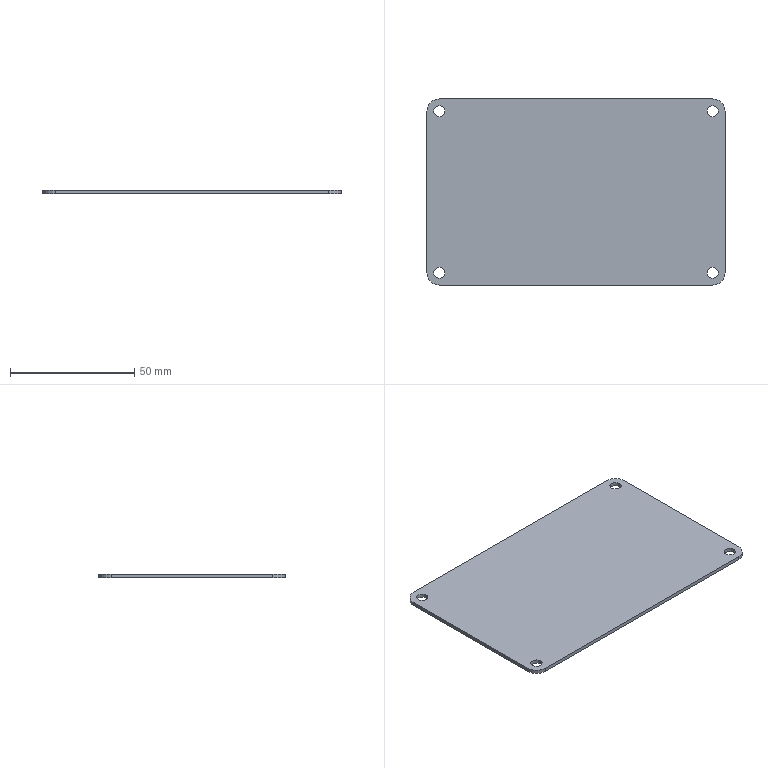Part | SolidWorks | features Fillet 1, FlatPattern 1, HoleWzd 1, SMBaseFlange 1, SheetMetal 1 | 1 solid | 18 faces | box 120 x 75 x 1.5 mm | volume 13372 mm3 | cylinder 12 | plane 6 | commonest cylinder face diameters 4.5 x8 10 x4
STEP:
#1=CARTESIAN_POINT('',(2.75,-5.,-1.5));
#2=VERTEX_POINT('',#1);
#3=CARTESIAN_POINT('',(7.25,-5.,-1.5));
#4=VERTEX_POINT('',#3);
#5=CARTESIAN_POINT('',(5.,-5.,-1.5));
#6=DIRECTION('',(0.,0.,1.));
#7=DIRECTION('',(1.,0.,0.));
#8=AXIS2_PLACEMENT_3D('',#5,#6,#7);
#9=CIRCLE('',#8,2.25);
#10=EDGE_CURVE('',#2,#4,#9,.T.);
#11=ORIENTED_EDGE('',*,*,#10,.F.);
#12=CARTESIAN_POINT('',(2.75,-5.,0.));
#13=VERTEX_POINT('',#12);
#14=CARTESIAN_POINT('',(2.75,-5.,0.));
#15=DIRECTION('',(0.,0.,1.));
#16=VECTOR('',#15,1000.);
#17=LINE('',#14,#16);
#18=EDGE_CURVE('',#2,#13,#17,.T.);
#19=ORIENTED_EDGE('',*,*,#18,.T.);
#20=CARTESIAN_POINT('',(7.25,-5.,0.));
#21=VERTEX_POINT('',#20);
#22=CARTESIAN_POINT('',(5.,-5.,0.));
#23=DIRECTION('',(0.,0.,1.));
#24=DIRECTION('',(1.,0.,0.));
#25=AXIS2_PLACEMENT_3D('',#22,#23,#24);
#26=CIRCLE('',#25,2.25);
#27=EDGE_CURVE('',#13,#21,#26,.T.);
#28=ORIENTED_EDGE('',*,*,#27,.T.);
#29=CARTESIAN_POINT('',(7.25,-5.,0.));
#30=DIRECTION('',(0.,0.,1.));
#31=VECTOR('',#30,1000.);
#32=LINE('',#29,#31);
#33=EDGE_CURVE('',#4,#21,#32,.T.);
#34=ORIENTED_EDGE('',*,*,#33,.F.);
#35=EDGE_LOOP('',(#11,#19,#28,#34));
#36=FACE_OUTER_BOUND('',#35,.T.);
#37=CARTESIAN_POINT('',(5.,-5.,0.));
#38=DIRECTION('',(0.,0.,1.));
#39=DIRECTION('',(1.,0.,0.));
#40=AXIS2_PLACEMENT_3D('',#37,#38,#39);
#41=CYLINDRICAL_SURFACE('',#40,2.25);
#42=ADVANCED_FACE('',(#36),#41,.F.);
#43=CARTESIAN_POINT('',(2.75,-70.,-1.5));
#44=VERTEX_POINT('',#43);
#45=CARTESIAN_POINT('',(7.25,-70.,-1.5));
#46=VERTEX_POINT('',#45);
#47=CARTESIAN_POINT('',(5.,-70.,-1.5));
#48=DIRECTION('',(0.,0.,1.));
#49=DIRECTION('',(1.,0.,0.));
#50=AXIS2_PLACEMENT_3D('',#47,#48,#49);
#51=CIRCLE('',#50,2.25);
#52=EDGE_CURVE('',#44,#46,#51,.T.);
#53=ORIENTED_EDGE('',*,*,#52,.F.);
#54=CARTESIAN_POINT('',(2.75,-70.,0.));
#55=VERTEX_POINT('',#54);
#56=CARTESIAN_POINT('',(2.75,-70.,0.));
#57=DIRECTION('',(0.,0.,1.));
#58=VECTOR('',#57,1000.);
#59=LINE('',#56,#58);
#60=EDGE_CURVE('',#44,#55,#59,.T.);
#61=ORIENTED_EDGE('',*,*,#60,.T.);
#62=CARTESIAN_POINT('',(7.25,-70.,0.));
#63=VERTEX_POINT('',#62);
#64=CARTESIAN_POINT('',(5.,-70.,0.));
#65=DIRECTION('',(0.,0.,1.));
#66=DIRECTION('',(1.,0.,0.));
#67=AXIS2_PLACEMENT_3D('',#64,#65,#66);
#68=CIRCLE('',#67,2.25);
#69=EDGE_CURVE('',#55,#63,#68,.T.);
#70=ORIENTED_EDGE('',*,*,#69,.T.);
#71=CARTESIAN_POINT('',(7.25,-70.,0.));
#72=DIRECTION('',(0.,0.,1.));
#73=VECTOR('',#72,1000.);
#74=LINE('',#71,#73);
#75=EDGE_CURVE('',#46,#63,#74,.T.);
#76=ORIENTED_EDGE('',*,*,#75,.F.);
#77=EDGE_LOOP('',(#53,#61,#70,#76));
#78=FACE_OUTER_BOUND('',#77,.T.);
#79=CARTESIAN_POINT('',(5.,-70.,0.));
#80=DIRECTION('',(0.,0.,1.));
#81=DIRECTION('',(1.,0.,0.));
#82=AXIS2_PLACEMENT_3D('',#79,#80,#81);
#83=CYLINDRICAL_SURFACE('',#82,2.25);
#84=ADVANCED_FACE('',(#78),#83,.F.);
#85=CARTESIAN_POINT('',(112.75,-70.,-1.5));
#86=VERTEX_POINT('',#85);
#87=CARTESIAN_POINT('',(117.25,-70.,-1.5));
#88=VERTEX_POINT('',#87);
#89=CARTESIAN_POINT('',(115.,-70.,-1.5));
#90=DIRECTION('',(0.,0.,1.));
#91=DIRECTION('',(1.,0.,0.));
#92=AXIS2_PLACEMENT_3D('',#89,#90,#91);
#93=CIRCLE('',#92,2.25);
#94=EDGE_CURVE('',#86,#88,#93,.T.);
#95=ORIENTED_EDGE('',*,*,#94,.F.);
#96=CARTESIAN_POINT('',(112.75,-70.,0.));
#97=VERTEX_POINT('',#96);
#98=CARTESIAN_POINT('',(112.75,-70.,0.));
#99=DIRECTION('',(0.,0.,1.));
#100=VECTOR('',#99,1000.);
#101=LINE('',#98,#100);
#102=EDGE_CURVE('',#86,#97,#101,.T.);
#103=ORIENTED_EDGE('',*,*,#102,.T.);
#104=CARTESIAN_POINT('',(117.25,-70.,0.));
#105=VERTEX_POINT('',#104);
#106=CARTESIAN_POINT('',(115.,-70.,0.));
#107=DIRECTION('',(0.,0.,1.));
#108=DIRECTION('',(1.,0.,0.));
#109=AXIS2_PLACEMENT_3D('',#106,#107,#108);
#110=CIRCLE('',#109,2.25);
#111=EDGE_CURVE('',#97,#105,#110,.T.);
#112=ORIENTED_EDGE('',*,*,#111,.T.);
#113=CARTESIAN_POINT('',(117.25,-70.,0.));
#114=DIRECTION('',(0.,0.,1.));
#115=VECTOR('',#114,1000.);
#116=LINE('',#113,#115);
#117=EDGE_CURVE('',#88,#105,#116,.T.);
#118=ORIENTED_EDGE('',*,*,#117,.F.);
#119=EDGE_LOOP('',(#95,#103,#112,#118));
#120=FACE_OUTER_BOUND('',#119,.T.);
#121=CARTESIAN_POINT('',(115.,-70.,0.));
#122=DIRECTION('',(0.,0.,1.));
#123=DIRECTION('',(1.,0.,0.));
#124=AXIS2_PLACEMENT_3D('',#121,#122,#123);
#125=CYLINDRICAL_SURFACE('',#124,2.25);
#126=ADVANCED_FACE('',(#120),#125,.F.);
#127=CARTESIAN_POINT('',(112.75,-5.,-1.5));
#128=VERTEX_POINT('',#127);
#129=CARTESIAN_POINT('',(117.25,-5.,-1.5));
#130=VERTEX_POINT('',#129);
#131=CARTESIAN_POINT('',(115.,-5.,-1.5));
#132=DIRECTION('',(0.,0.,1.));
#133=DIRECTION('',(1.,0.,0.));
#134=AXIS2_PLACEMENT_3D('',#131,#132,#133);
#135=CIRCLE('',#134,2.25);
#136=EDGE_CURVE('',#128,#130,#135,.T.);
#137=ORIENTED_EDGE('',*,*,#136,.F.);
#138=CARTESIAN_POINT('',(112.75,-5.,0.));
#139=VERTEX_POINT('',#138);
#140=CARTESIAN_POINT('',(112.75,-5.,0.));
#141=DIRECTION('',(0.,0.,1.));
#142=VECTOR('',#141,1000.);
#143=LINE('',#140,#142);
#144=EDGE_CURVE('',#128,#139,#143,.T.);
#145=ORIENTED_EDGE('',*,*,#144,.T.);
#146=CARTESIAN_POINT('',(117.25,-5.,0.));
#147=VERTEX_POINT('',#146);
#148=CARTESIAN_POINT('',(115.,-5.,0.));
#149=DIRECTION('',(0.,0.,1.));
#150=DIRECTION('',(1.,0.,0.));
#151=AXIS2_PLACEMENT_3D('',#148,#149,#150);
#152=CIRCLE('',#151,2.25);
#153=EDGE_CURVE('',#139,#147,#152,.T.);
#154=ORIENTED_EDGE('',*,*,#153,.T.);
#155=CARTESIAN_POINT('',(117.25,-5.,0.));
#156=DIRECTION('',(0.,0.,1.));
#157=VECTOR('',#156,1000.);
#158=LINE('',#155,#157);
#159=EDGE_CURVE('',#130,#147,#158,.T.);
#160=ORIENTED_EDGE('',*,*,#159,.F.);
#161=EDGE_LOOP('',(#137,#145,#154,#160));
#162=FACE_OUTER_BOUND('',#161,.T.);
#163=CARTESIAN_POINT('',(115.,-5.,0.));
#164=DIRECTION('',(0.,0.,1.));
#165=DIRECTION('',(1.,0.,0.));
#166=AXIS2_PLACEMENT_3D('',#163,#164,#165);
#167=CYLINDRICAL_SURFACE('',#166,2.25);
#168=ADVANCED_FACE('',(#162),#167,.F.);
#169=CARTESIAN_POINT('',(0.,-5.,-1.5));
#170=VERTEX_POINT('',#169);
#171=CARTESIAN_POINT('',(0.,-70.,-1.5));
#172=VERTEX_POINT('',#171);
#173=CARTESIAN_POINT('',(0.,0.,-1.5));
#174=DIRECTION('',(0.,-1.,0.));
#175=VECTOR('',#174,1000.);
#176=LINE('',#173,#175);
#177=EDGE_CURVE('',#170,#172,#176,.T.);
#178=ORIENTED_EDGE('',*,*,#177,.T.);
#179=CARTESIAN_POINT('',(0.,-70.,0.));
#180=VERTEX_POINT('',#179);
#181=CARTESIAN_POINT('',(0.,-70.,-1.5));
#182=DIRECTION('',(0.,0.,1.));
#183=VECTOR('',#182,1000.);
#184=LINE('',#181,#183);
#185=EDGE_CURVE('',#172,#180,#184,.T.);
#186=ORIENTED_EDGE('',*,*,#185,.T.);
#187=CARTESIAN_POINT('',(0.,-5.,0.));
#188=VERTEX_POINT('',#187);
#189=CARTESIAN_POINT('',(0.,0.,0.));
#190=DIRECTION('',(0.,-1.,0.));
#191=VECTOR('',#190,1000.);
#192=LINE('',#189,#191);
#193=EDGE_CURVE('',#188,#180,#192,.T.);
#194=ORIENTED_EDGE('',*,*,#193,.F.);
#195=CARTESIAN_POINT('',(0.,-5.,-1.5));
#196=DIRECTION('',(0.,0.,-1.));
#197=VECTOR('',#196,1000.);
#198=LINE('',#195,#197);
#199=EDGE_CURVE('',#188,#170,#198,.T.);
#200=ORIENTED_EDGE('',*,*,#199,.T.);
#201=EDGE_LOOP('',(#178,#186,#194,#200));
#202=FACE_OUTER_BOUND('',#201,.T.);
#203=CARTESIAN_POINT('',(0.,0.,-1.5));
#204=DIRECTION('',(-1.,0.,0.));
#205=DIRECTION('',(0.,-1.,0.));
#206=AXIS2_PLACEMENT_3D('',#203,#204,#205);
#207=PLANE('',#206);
#208=ADVANCED_FACE('',(#202),#207,.T.);
#209=CARTESIAN_POINT('',(115.,0.,0.));
#210=VERTEX_POINT('',#209);
#211=CARTESIAN_POINT('',(5.,0.,0.));
#212=VERTEX_POINT('',#211);
#213=CARTESIAN_POINT('',(0.,0.,0.));
#214=DIRECTION('',(-1.,0.,0.));
#215=VECTOR('',#214,1000.);
#216=LINE('',#213,#215);
#217=EDGE_CURVE('',#210,#212,#216,.T.);
#218=ORIENTED_EDGE('',*,*,#217,.F.);
#219=CARTESIAN_POINT('',(115.,0.,-1.5));
#220=VERTEX_POINT('',#219);
#221=CARTESIAN_POINT('',(115.,0.,-1.5));
#222=DIRECTION('',(0.,0.,-1.));
#223=VECTOR('',#222,1000.);
#224=LINE('',#221,#223);
#225=EDGE_CURVE('',#210,#220,#224,.T.);
#226=ORIENTED_EDGE('',*,*,#225,.T.);
#227=CARTESIAN_POINT('',(5.,0.,-1.5));
#228=VERTEX_POINT('',#227);
#229=CARTESIAN_POINT('',(0.,0.,-1.5));
#230=DIRECTION('',(-1.,0.,0.));
#231=VECTOR('',#230,1000.);
#232=LINE('',#229,#231);
#233=EDGE_CURVE('',#220,#228,#232,.T.);
#234=ORIENTED_EDGE('',*,*,#233,.T.);
#235=CARTESIAN_POINT('',(5.,0.,-1.5));
#236=DIRECTION('',(0.,0.,1.));
#237=VECTOR('',#236,1000.);
#238=LINE('',#235,#237);
#239=EDGE_CURVE('',#228,#212,#238,.T.);
#240=ORIENTED_EDGE('',*,*,#239,.T.);
#241=EDGE_LOOP('',(#218,#226,#234,#240));
#242=FACE_OUTER_BOUND('',#241,.T.);
#243=CARTESIAN_POINT('',(0.,0.,-1.5));
#244=DIRECTION('',(0.,1.,0.));
#245=DIRECTION('',(0.,0.,1.));
#246=AXIS2_PLACEMENT_3D('',#243,#244,#245);
#247=PLANE('',#246);
#248=ADVANCED_FACE('',(#242),#247,.T.);
#249=CARTESIAN_POINT('',(120.,-70.,0.));
#250=VERTEX_POINT('',#249);
#251=CARTESIAN_POINT('',(120.,-5.,0.));
#252=VERTEX_POINT('',#251);
#253=CARTESIAN_POINT('',(120.,0.,0.));
#254=DIRECTION('',(0.,1.,0.));
#255=VECTOR('',#254,1000.);
#256=LINE('',#253,#255);
#257=EDGE_CURVE('',#250,#252,#256,.T.);
#258=ORIENTED_EDGE('',*,*,#257,.F.);
#259=CARTESIAN_POINT('',(120.,-70.,-1.5));
#260=VERTEX_POINT('',#259);
#261=CARTESIAN_POINT('',(120.,-70.,-1.5));
#262=DIRECTION('',(0.,0.,-1.));
#263=VECTOR('',#262,1000.);
#264=LINE('',#261,#263);
#265=EDGE_CURVE('',#250,#260,#264,.T.);
#266=ORIENTED_EDGE('',*,*,#265,.T.);
#267=CARTESIAN_POINT('',(120.,-5.,-1.5));
#268=VERTEX_POINT('',#267);
#269=CARTESIAN_POINT('',(120.,0.,-1.5));
#270=DIRECTION('',(0.,1.,0.));
#271=VECTOR('',#270,1000.);
#272=LINE('',#269,#271);
#273=EDGE_CURVE('',#260,#268,#272,.T.);
#274=ORIENTED_EDGE('',*,*,#273,.T.);
#275=CARTESIAN_POINT('',(120.,-5.,-1.5));
#276=DIRECTION('',(0.,0.,1.));
#277=VECTOR('',#276,1000.);
#278=LINE('',#275,#277);
#279=EDGE_CURVE('',#268,#252,#278,.T.);
#280=ORIENTED_EDGE('',*,*,#279,.T.);
#281=EDGE_LOOP('',(#258,#266,#274,#280));
#282=FACE_OUTER_BOUND('',#281,.T.);
#283=CARTESIAN_POINT('',(120.,0.,-1.5));
#284=DIRECTION('',(1.,0.,0.));
#285=DIRECTION('',(0.,1.,0.));
#286=AXIS2_PLACEMENT_3D('',#283,#284,#285);
#287=PLANE('',#286);
#288=ADVANCED_FACE('',(#282),#287,.T.);
#289=CARTESIAN_POINT('',(5.,-75.,0.));
#290=VERTEX_POINT('',#289);
#291=CARTESIAN_POINT('',(115.,-75.,0.));
#292=VERTEX_POINT('',#291);
#293=CARTESIAN_POINT('',(0.,-75.,0.));
#294=DIRECTION('',(1.,0.,0.));
#295=VECTOR('',#294,1000.);
#296=LINE('',#293,#295);
#297=EDGE_CURVE('',#290,#292,#296,.T.);
#298=ORIENTED_EDGE('',*,*,#297,.F.);
#299=CARTESIAN_POINT('',(5.,-75.,-1.5));
#300=VERTEX_POINT('',#299);
#301=CARTESIAN_POINT('',(5.,-75.,-1.5));
#302=DIRECTION('',(0.,0.,-1.));
#303=VECTOR('',#302,1000.);
#304=LINE('',#301,#303);
#305=EDGE_CURVE('',#290,#300,#304,.T.);
#306=ORIENTED_EDGE('',*,*,#305,.T.);
#307=CARTESIAN_POINT('',(115.,-75.,-1.5));
#308=VERTEX_POINT('',#307);
#309=CARTESIAN_POINT('',(0.,-75.,-1.5));
#310=DIRECTION('',(1.,0.,0.));
#311=VECTOR('',#310,1000.);
#312=LINE('',#309,#311);
#313=EDGE_CURVE('',#300,#308,#312,.T.);
#314=ORIENTED_EDGE('',*,*,#313,.T.);
#315=CARTESIAN_POINT('',(115.,-75.,-1.5));
#316=DIRECTION('',(0.,0.,1.));
#317=VECTOR('',#316,1000.);
#318=LINE('',#315,#317);
#319=EDGE_CURVE('',#308,#292,#318,.T.);
#320=ORIENTED_EDGE('',*,*,#319,.T.);
#321=EDGE_LOOP('',(#298,#306,#314,#320));
#322=FACE_OUTER_BOUND('',#321,.T.);
#323=CARTESIAN_POINT('',(0.,-75.,-1.5));
#324=DIRECTION('',(0.,-1.,0.));
#325=DIRECTION('',(0.,0.,-1.));
#326=AXIS2_PLACEMENT_3D('',#323,#324,#325);
#327=PLANE('',#326);
#328=ADVANCED_FACE('',(#322),#327,.T.);
#329=CARTESIAN_POINT('',(5.,-5.,-1.5));
#330=DIRECTION('',(0.,0.,1.));
#331=DIRECTION('',(1.,0.,0.));
#332=AXIS2_PLACEMENT_3D('',#329,#330,#331);
#333=CIRCLE('',#332,2.25);
#334=EDGE_CURVE('',#4,#2,#333,.T.);
#335=ORIENTED_EDGE('',*,*,#334,.T.);
#336=ORIENTED_EDGE('',*,*,#10,.T.);
#337=EDGE_LOOP('',(#335,#336));
#338=FACE_BOUND('',#337,.T.);
#339=CARTESIAN_POINT('',(5.,-70.,-1.5));
#340=DIRECTION('',(0.,0.,1.));
#341=DIRECTION('',(1.,0.,0.));
#342=AXIS2_PLACEMENT_3D('',#339,#340,#341);
#343=CIRCLE('',#342,2.25);
#344=EDGE_CURVE('',#46,#44,#343,.T.);
#345=ORIENTED_EDGE('',*,*,#344,.T.);
#346=ORIENTED_EDGE('',*,*,#52,.T.);
#347=EDGE_LOOP('',(#345,#346));
#348=FACE_BOUND('',#347,.T.);
#349=CARTESIAN_POINT('',(115.,-70.,-1.5));
#350=DIRECTION('',(0.,0.,1.));
#351=DIRECTION('',(1.,0.,0.));
#352=AXIS2_PLACEMENT_3D('',#349,#350,#351);
#353=CIRCLE('',#352,2.25);
#354=EDGE_CURVE('',#88,#86,#353,.T.);
#355=ORIENTED_EDGE('',*,*,#354,.T.);
#356=ORIENTED_EDGE('',*,*,#94,.T.);
#357=EDGE_LOOP('',(#355,#356));
#358=FACE_BOUND('',#357,.T.);
#359=CARTESIAN_POINT('',(115.,-5.,-1.5));
#360=DIRECTION('',(0.,0.,1.));
#361=DIRECTION('',(1.,0.,0.));
#362=AXIS2_PLACEMENT_3D('',#359,#360,#361);
#363=CIRCLE('',#362,2.25);
#364=EDGE_CURVE('',#130,#128,#363,.T.);
#365=ORIENTED_EDGE('',*,*,#364,.T.);
#366=ORIENTED_EDGE('',*,*,#136,.T.);
#367=EDGE_LOOP('',(#365,#366));
#368=FACE_BOUND('',#367,.T.);
#369=ORIENTED_EDGE('',*,*,#313,.F.);
#370=CARTESIAN_POINT('',(5.,-70.,-1.5));
#371=DIRECTION('',(0.,0.,-1.));
#372=DIRECTION('',(1.,0.,0.));
#373=AXIS2_PLACEMENT_3D('',#370,#371,#372);
#374=CIRCLE('',#373,5.);
#375=EDGE_CURVE('',#300,#172,#374,.T.);
#376=ORIENTED_EDGE('',*,*,#375,.T.);
#377=ORIENTED_EDGE('',*,*,#177,.F.);
#378=CARTESIAN_POINT('',(5.,-5.,-1.5));
#379=DIRECTION('',(0.,0.,-1.));
#380=DIRECTION('',(1.,0.,0.));
#381=AXIS2_PLACEMENT_3D('',#378,#379,#380);
#382=CIRCLE('',#381,5.);
#383=EDGE_CURVE('',#170,#228,#382,.T.);
#384=ORIENTED_EDGE('',*,*,#383,.T.);
#385=ORIENTED_EDGE('',*,*,#233,.F.);
#386=CARTESIAN_POINT('',(115.,-5.,-1.5));
#387=DIRECTION('',(0.,0.,-1.));
#388=DIRECTION('',(1.,0.,0.));
#389=AXIS2_PLACEMENT_3D('',#386,#387,#388);
#390=CIRCLE('',#389,5.);
#391=EDGE_CURVE('',#220,#268,#390,.T.);
#392=ORIENTED_EDGE('',*,*,#391,.T.);
#393=ORIENTED_EDGE('',*,*,#273,.F.);
#394=CARTESIAN_POINT('',(115.,-70.,-1.5));
#395=DIRECTION('',(0.,0.,-1.));
#396=DIRECTION('',(1.,0.,0.));
#397=AXIS2_PLACEMENT_3D('',#394,#395,#396);
#398=CIRCLE('',#397,5.);
#399=EDGE_CURVE('',#260,#308,#398,.T.);
#400=ORIENTED_EDGE('',*,*,#399,.T.);
#401=EDGE_LOOP('',(#369,#376,#377,#384,#385,#392,#393,#400));
#402=FACE_OUTER_BOUND('',#401,.T.);
#403=CARTESIAN_POINT('',(0.,0.,-1.5));
#404=DIRECTION('',(0.,0.,1.));
#405=DIRECTION('',(1.,0.,0.));
#406=AXIS2_PLACEMENT_3D('',#403,#404,#405);
#407=PLANE('',#406);
#408=ADVANCED_FACE('',(#338,#348,#358,#368,#402),#407,.F.);
#409=CARTESIAN_POINT('',(5.,-5.,0.));
#410=DIRECTION('',(0.,0.,1.));
#411=DIRECTION('',(1.,0.,0.));
#412=AXIS2_PLACEMENT_3D('',#409,#410,#411);
#413=CIRCLE('',#412,2.25);
#414=EDGE_CURVE('',#21,#13,#413,.T.);
#415=ORIENTED_EDGE('',*,*,#414,.F.);
#416=ORIENTED_EDGE('',*,*,#27,.F.);
#417=EDGE_LOOP('',(#415,#416));
#418=FACE_BOUND('',#417,.T.);
#419=CARTESIAN_POINT('',(5.,-70.,0.));
#420=DIRECTION('',(0.,0.,1.));
#421=DIRECTION('',(1.,0.,0.));
#422=AXIS2_PLACEMENT_3D('',#419,#420,#421);
#423=CIRCLE('',#422,2.25);
#424=EDGE_CURVE('',#63,#55,#423,.T.);
#425=ORIENTED_EDGE('',*,*,#424,.F.);
#426=ORIENTED_EDGE('',*,*,#69,.F.);
#427=EDGE_LOOP('',(#425,#426));
#428=FACE_BOUND('',#427,.T.);
#429=CARTESIAN_POINT('',(115.,-70.,0.));
#430=DIRECTION('',(0.,0.,1.));
#431=DIRECTION('',(1.,0.,0.));
#432=AXIS2_PLACEMENT_3D('',#429,#430,#431);
#433=CIRCLE('',#432,2.25);
#434=EDGE_CURVE('',#105,#97,#433,.T.);
#435=ORIENTED_EDGE('',*,*,#434,.F.);
#436=ORIENTED_EDGE('',*,*,#111,.F.);
#437=EDGE_LOOP('',(#435,#436));
#438=FACE_BOUND('',#437,.T.);
#439=CARTESIAN_POINT('',(115.,-5.,0.));
#440=DIRECTION('',(0.,0.,1.));
#441=DIRECTION('',(1.,0.,0.));
#442=AXIS2_PLACEMENT_3D('',#439,#440,#441);
#443=CIRCLE('',#442,2.25);
#444=EDGE_CURVE('',#147,#139,#443,.T.);
#445=ORIENTED_EDGE('',*,*,#444,.F.);
#446=ORIENTED_EDGE('',*,*,#153,.F.);
#447=EDGE_LOOP('',(#445,#446));
#448=FACE_BOUND('',#447,.T.);
#449=ORIENTED_EDGE('',*,*,#193,.T.);
#450=CARTESIAN_POINT('',(5.,-70.,0.));
#451=DIRECTION('',(0.,0.,1.));
#452=DIRECTION('',(1.,0.,0.));
#453=AXIS2_PLACEMENT_3D('',#450,#451,#452);
#454=CIRCLE('',#453,5.);
#455=EDGE_CURVE('',#180,#290,#454,.T.);
#456=ORIENTED_EDGE('',*,*,#455,.T.);
#457=ORIENTED_EDGE('',*,*,#297,.T.);
#458=CARTESIAN_POINT('',(115.,-70.,0.));
#459=DIRECTION('',(0.,0.,1.));
#460=DIRECTION('',(1.,0.,0.));
#461=AXIS2_PLACEMENT_3D('',#458,#459,#460);
#462=CIRCLE('',#461,5.);
#463=EDGE_CURVE('',#292,#250,#462,.T.);
#464=ORIENTED_EDGE('',*,*,#463,.T.);
#465=ORIENTED_EDGE('',*,*,#257,.T.);
#466=CARTESIAN_POINT('',(115.,-5.,0.));
#467=DIRECTION('',(0.,0.,1.));
#468=DIRECTION('',(1.,0.,0.));
#469=AXIS2_PLACEMENT_3D('',#466,#467,#468);
#470=CIRCLE('',#469,5.);
#471=EDGE_CURVE('',#252,#210,#470,.T.);
#472=ORIENTED_EDGE('',*,*,#471,.T.);
#473=ORIENTED_EDGE('',*,*,#217,.T.);
#474=CARTESIAN_POINT('',(5.,-5.,0.));
#475=DIRECTION('',(0.,0.,1.));
#476=DIRECTION('',(1.,0.,0.));
#477=AXIS2_PLACEMENT_3D('',#474,#475,#476);
#478=CIRCLE('',#477,5.);
#479=EDGE_CURVE('',#212,#188,#478,.T.);
#480=ORIENTED_EDGE('',*,*,#479,.T.);
#481=EDGE_LOOP('',(#449,#456,#457,#464,#465,#472,#473,#480));
#482=FACE_OUTER_BOUND('',#481,.T.);
#483=CARTESIAN_POINT('',(0.,0.,0.));
#484=DIRECTION('',(0.,0.,1.));
#485=DIRECTION('',(1.,0.,0.));
#486=AXIS2_PLACEMENT_3D('',#483,#484,#485);
#487=PLANE('',#486);
#488=ADVANCED_FACE('',(#418,#428,#438,#448,#482),#487,.T.);
#489=ORIENTED_EDGE('',*,*,#375,.F.);
#490=ORIENTED_EDGE('',*,*,#305,.F.);
#491=ORIENTED_EDGE('',*,*,#455,.F.);
#492=ORIENTED_EDGE('',*,*,#185,.F.);
#493=EDGE_LOOP('',(#489,#490,#491,#492));
#494=FACE_OUTER_BOUND('',#493,.T.);
#495=CARTESIAN_POINT('',(5.,-70.,-1.5));
#496=DIRECTION('',(0.,0.,1.));
#497=DIRECTION('',(1.,0.,0.));
#498=AXIS2_PLACEMENT_3D('',#495,#496,#497);
#499=CYLINDRICAL_SURFACE('',#498,5.);
#500=ADVANCED_FACE('',(#494),#499,.T.);
#501=ORIENTED_EDGE('',*,*,#399,.F.);
#502=ORIENTED_EDGE('',*,*,#265,.F.);
#503=ORIENTED_EDGE('',*,*,#463,.F.);
#504=ORIENTED_EDGE('',*,*,#319,.F.);
#505=EDGE_LOOP('',(#501,#502,#503,#504));
#506=FACE_OUTER_BOUND('',#505,.T.);
#507=CARTESIAN_POINT('',(115.,-70.,-1.5));
#508=DIRECTION('',(0.,0.,1.));
#509=DIRECTION('',(1.,0.,0.));
#510=AXIS2_PLACEMENT_3D('',#507,#508,#509);
#511=CYLINDRICAL_SURFACE('',#510,5.);
#512=ADVANCED_FACE('',(#506),#511,.T.);
#513=ORIENTED_EDGE('',*,*,#391,.F.);
#514=ORIENTED_EDGE('',*,*,#225,.F.);
#515=ORIENTED_EDGE('',*,*,#471,.F.);
#516=ORIENTED_EDGE('',*,*,#279,.F.);
#517=EDGE_LOOP('',(#513,#514,#515,#516));
#518=FACE_OUTER_BOUND('',#517,.T.);
#519=CARTESIAN_POINT('',(115.,-5.,-1.5));
#520=DIRECTION('',(0.,0.,1.));
#521=DIRECTION('',(1.,0.,0.));
#522=AXIS2_PLACEMENT_3D('',#519,#520,#521);
#523=CYLINDRICAL_SURFACE('',#522,5.);
#524=ADVANCED_FACE('',(#518),#523,.T.);
#525=ORIENTED_EDGE('',*,*,#383,.F.);
#526=ORIENTED_EDGE('',*,*,#199,.F.);
#527=ORIENTED_EDGE('',*,*,#479,.F.);
#528=ORIENTED_EDGE('',*,*,#239,.F.);
#529=EDGE_LOOP('',(#525,#526,#527,#528));
#530=FACE_OUTER_BOUND('',#529,.T.);
#531=CARTESIAN_POINT('',(5.,-5.,-1.5));
#532=DIRECTION('',(0.,0.,1.));
#533=DIRECTION('',(1.,0.,0.));
#534=AXIS2_PLACEMENT_3D('',#531,#532,#533);
#535=CYLINDRICAL_SURFACE('',#534,5.);
#536=ADVANCED_FACE('',(#530),#535,.T.);
#537=ORIENTED_EDGE('',*,*,#144,.F.);
#538=ORIENTED_EDGE('',*,*,#364,.F.);
#539=ORIENTED_EDGE('',*,*,#159,.T.);
#540=ORIENTED_EDGE('',*,*,#444,.T.);
#541=EDGE_LOOP('',(#537,#538,#539,#540));
#542=FACE_OUTER_BOUND('',#541,.T.);
#543=CARTESIAN_POINT('',(115.,-5.,0.));
#544=DIRECTION('',(0.,0.,1.));
#545=DIRECTION('',(1.,0.,0.));
#546=AXIS2_PLACEMENT_3D('',#543,#544,#545);
#547=CYLINDRICAL_SURFACE('',#546,2.25);
#548=ADVANCED_FACE('',(#542),#547,.F.);
#549=ORIENTED_EDGE('',*,*,#102,.F.);
#550=ORIENTED_EDGE('',*,*,#354,.F.);
#551=ORIENTED_EDGE('',*,*,#117,.T.);
#552=ORIENTED_EDGE('',*,*,#434,.T.);
#553=EDGE_LOOP('',(#549,#550,#551,#552));
#554=FACE_OUTER_BOUND('',#553,.T.);
#555=CARTESIAN_POINT('',(115.,-70.,0.));
#556=DIRECTION('',(0.,0.,1.));
#557=DIRECTION('',(1.,0.,0.));
#558=AXIS2_PLACEMENT_3D('',#555,#556,#557);
#559=CYLINDRICAL_SURFACE('',#558,2.25);
#560=ADVANCED_FACE('',(#554),#559,.F.);
#561=ORIENTED_EDGE('',*,*,#60,.F.);
#562=ORIENTED_EDGE('',*,*,#344,.F.);
#563=ORIENTED_EDGE('',*,*,#75,.T.);
#564=ORIENTED_EDGE('',*,*,#424,.T.);
#565=EDGE_LOOP('',(#561,#562,#563,#564));
#566=FACE_OUTER_BOUND('',#565,.T.);
#567=CARTESIAN_POINT('',(5.,-70.,0.));
#568=DIRECTION('',(0.,0.,1.));
#569=DIRECTION('',(1.,0.,0.));
#570=AXIS2_PLACEMENT_3D('',#567,#568,#569);
#571=CYLINDRICAL_SURFACE('',#570,2.25);
#572=ADVANCED_FACE('',(#566),#571,.F.);
#573=ORIENTED_EDGE('',*,*,#18,.F.);
#574=ORIENTED_EDGE('',*,*,#334,.F.);
#575=ORIENTED_EDGE('',*,*,#33,.T.);
#576=ORIENTED_EDGE('',*,*,#414,.T.);
#577=EDGE_LOOP('',(#573,#574,#575,#576));
#578=FACE_OUTER_BOUND('',#577,.T.);
#579=CARTESIAN_POINT('',(5.,-5.,0.));
#580=DIRECTION('',(0.,0.,1.));
#581=DIRECTION('',(1.,0.,0.));
#582=AXIS2_PLACEMENT_3D('',#579,#580,#581);
#583=CYLINDRICAL_SURFACE('',#582,2.25);
#584=ADVANCED_FACE('',(#578),#583,.F.);
#585=CLOSED_SHELL('',(#42,#84,#126,#168,#208,#248,#288,#328,#408,#488,#500,#512,#524,#536,#548,#560,#572,#584));
#586=MANIFOLD_SOLID_BREP('',#585);
#587=CARTESIAN_POINT('',(0.,0.,0.));
#588=DIRECTION('',(0.,0.,1.));
#589=DIRECTION('',(1.,0.,0.));
#590=AXIS2_PLACEMENT_3D('',#587,#588,#589);
#591=(LENGTH_UNIT()NAMED_UNIT(*)SI_UNIT(.MILLI.,.METRE.));
#592=UNCERTAINTY_MEASURE_WITH_UNIT(LENGTH_MEASURE(0.00001),#591,'','');
#593=(NAMED_UNIT(*)PLANE_ANGLE_UNIT()SI_UNIT($,.RADIAN.));
#594=(NAMED_UNIT(*)SI_UNIT($,.STERADIAN.)SOLID_ANGLE_UNIT());
#595=(GEOMETRIC_REPRESENTATION_CONTEXT(3)GLOBAL_UNCERTAINTY_ASSIGNED_CONTEXT((#592))GLOBAL_UNIT_ASSIGNED_CONTEXT((#591,#593,#594))REPRESENTATION_CONTEXT('',''));
#596=ADVANCED_BREP_SHAPE_REPRESENTATION('',(#586,#590),#595);